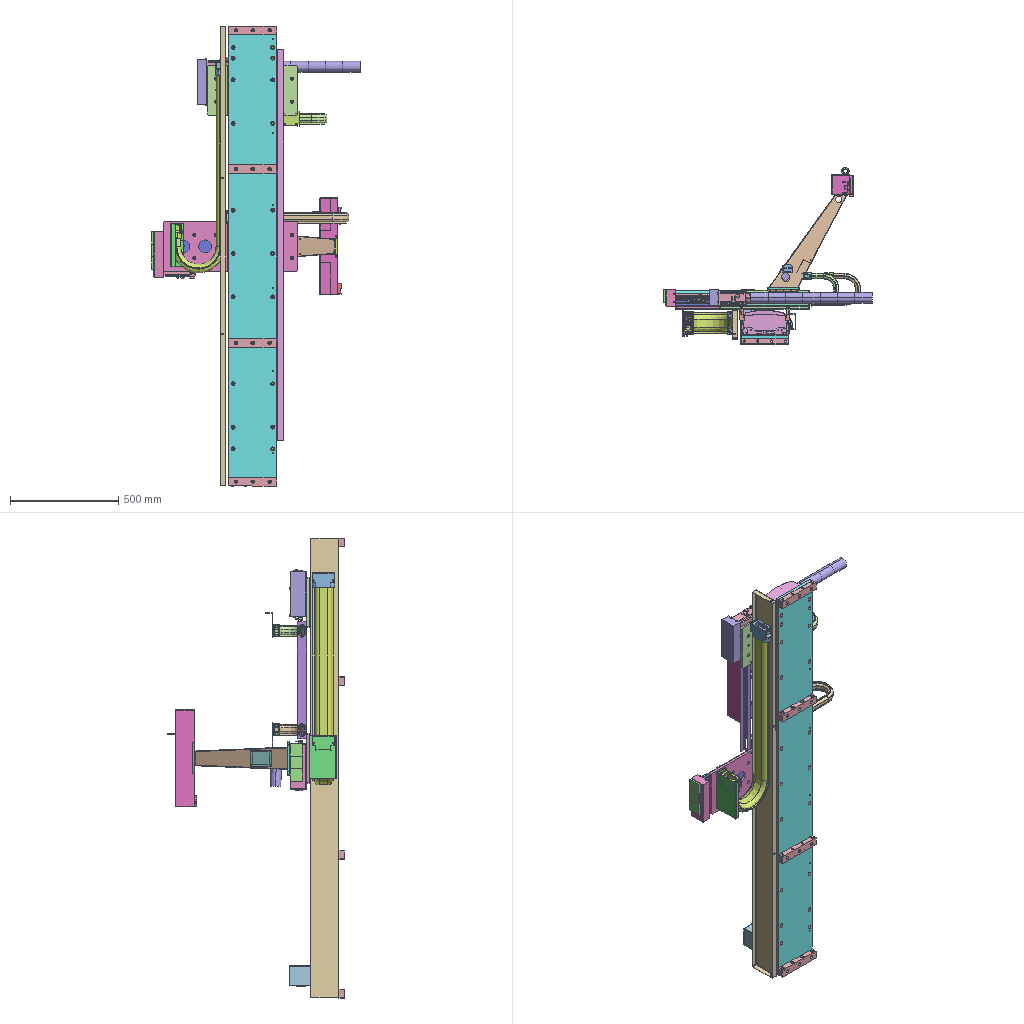Assembly | SolidWorks | 80 different items | 115 placed | box 960 x 815 x 2120 mm
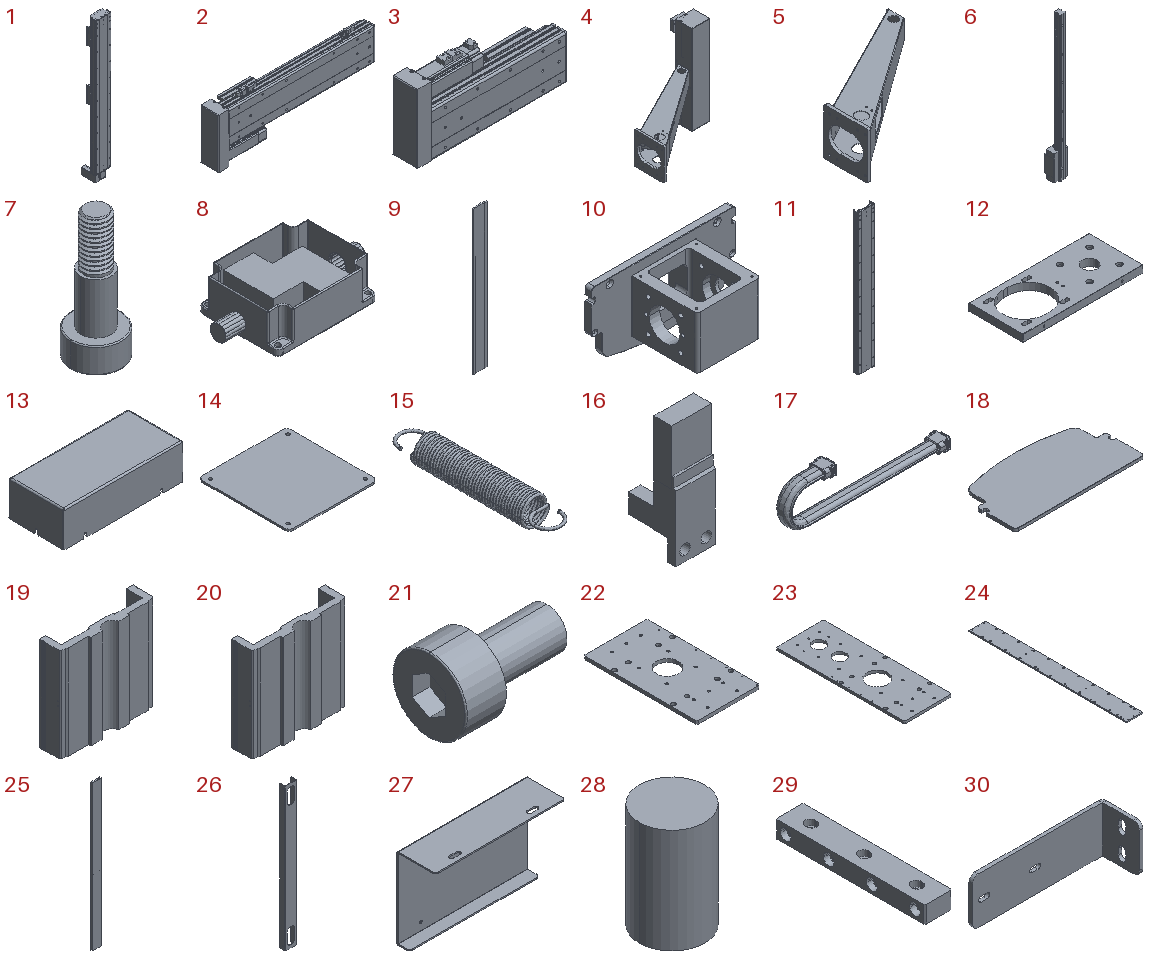Parts list (item | name | quantity | parent item | size | volume | features):
1 | (subassembly) | x1 | - | 242 x 213.35 x 2015 mm | 19740155 mm3 | -
2 | (subassembly) | x1 | - | 660 x 78 x 229.35 mm | 4358113 mm3 | -
3 | (subassembly) | x1 | - | 460 x 78 x 235.85 mm | 3440489 mm3 | -
4 | (subassembly) | x1 | - | 562.593 x 396.277 x 446 mm | 1438973 mm3 | -
5 | (subassembly) | x1 | in 4 | 438.467 x 369.277 x 160 mm | 471862 mm3 | -
6 | (subassembly) | x1 | in 4 | 34 x 28 x 350 mm | 100093 mm3 | -
7 | - | x1 | in 4 | 10 x 10 x 25 mm | 739.596 mm3 | features ICE 3, Chamfer 1, Extrusion 1, Fillet 1, SweepThread 1
8 | - | x1 | in 4 | 140 x 80 x 36 mm | 91649 mm3 | features Boss 2, Cut 2, Extrusion 1, Fillet 1, LPattern 1, Shell 1
9 | - | x1 | in 1 | 188.037 x 25 x 1900 mm | 6268934 mm3 | features BaseBody 1
10 | - | x1 | in 1 | 220 x 126 x 113.5 mm | 568343 mm3 | features BaseBody 1
11 | - | x1 | in 1 | 220 x 67.5 x 1900 mm | 10276544 mm3 | features BaseBody 1
12 | - | x1 | in 1 | 200 x 90 x 12 mm | 145701 mm3 | features BaseBody 1
13 | - | x1 | in 1 | 203.7 x 93.7 x 60.5 mm | 79662 mm3 | features BaseBody 1
14 | - | x2 | in 1 | 97 x 100 x 2 mm | 19276 mm3 | features BaseBody 1
15 | - | x1 | in 4 | 6.01 x 35.7 x 6.018 mm | 209.96 mm3 | features BaseBody 83
16 | - | x4 | in 1 | 13 x 15.5 x 39.5 mm | 3396 mm3 | features BaseBody 2
17 | - | x1 | - | 573.5 x 56 x 153.4 mm | 269954 mm3 | features BaseBody 3
18 | - | x1 | in 1 | 220 x 113.5 x 5 mm | 112175 mm3 | features BaseBody 1
19 | - | x1 | in 1 | 230 x 60 x 230 mm | 1114980 mm3 | features BaseBody 1
20 | - | x1 | in 1 | 230 x 60 x 230 mm | 1114980 mm3 | features BaseBody 1
21 | - | x14 | in 1 | 9 x 5.5 x 5.5 mm | 106.321 mm3 | features BaseBody 1
22 | - | x1 | - | 230 x 415 x 12 mm | 1051466 mm3 | features HoleWzd 5, Chamfer 1, Extrusion 1, ICE 1
23 | - | x1 | - | 230 x 616 x 12 mm | 1500608 mm3 | features HoleWzd 6, Chamfer 1, Extrusion 1, ICE 1
24 | - | x1 | - | 220 x 2115 x 15 mm | 6896303 mm3 | features HoleWzd 3, Chamfer 1, Extrusion 1
25 | - | x1 | - | 132 x 25 x 2116 mm | 573342 mm3 | features ICE 2, EdgeFlange 1, FlatPattern 1, HoleWzd 1, SMBaseFlange 1, SheetMetal 1
26 | - | x1 | - | 43 x 21.5 x 540 mm | 61599 mm3 | features Cut 1, Fillet 1, FlatPattern 1, HoleWzd 1, SMBaseFlange 1, SheetMetal 1
27 | - | x1 | - | 200 x 60 x 125 mm | 79463 mm3 | features Fillet 1, FlatPattern 1, HoleWzd 1, ICE 1, SMBaseFlange 1, SheetMetal 1
28 | - | x8 | - | 50 x 50 x 80 mm | 157080 mm3 | features Extrusion 1
29 | - | x4 | - | 40 x 220 x 25 mm | 193089 mm3 | features HoleWzd 2, Chamfer 1, Extrusion 1
30 | - | x2 | - | 115 x 35 x 40 mm | 16866 mm3 | features ICE 2, Fillet 1, FlatPattern 1, HoleWzd 1, SMBaseFlange 1, SheetMetal 1
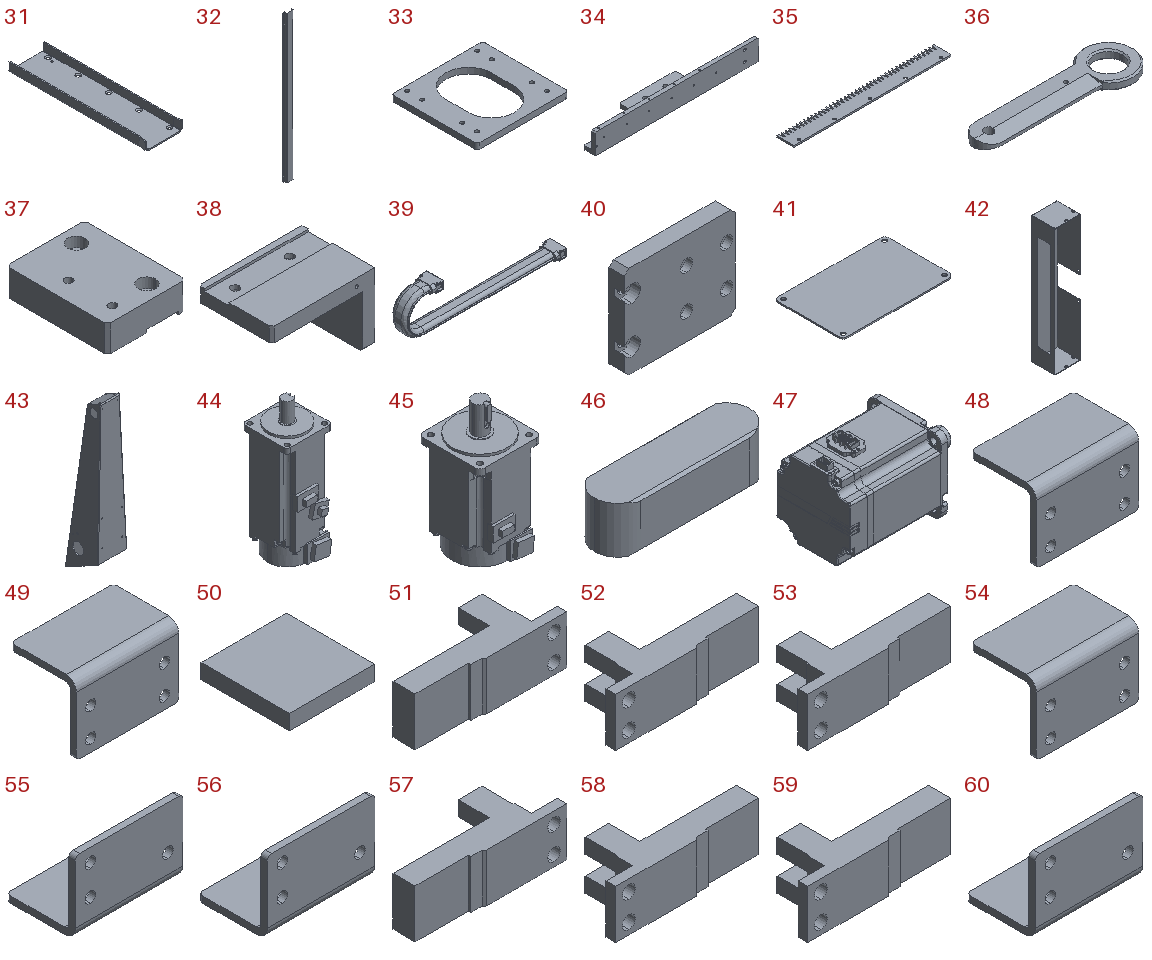31 | - | x2 | - | 69.801 x 254 x 16 mm | 45736 mm3 | features EdgeFlange 2, HoleWzd 2, Fillet 1, FlatPattern 1, ICE 1, SMBaseFlange 1, SheetMetal 1
32 | - | x1 | - | 92 x 32 x 1800 mm | 504480 mm3 | features Fillet 1, FlatPattern 1, ICE 1, SMBaseFlange 1, SheetMetal 1
33 | - | x1 | in 5 | 160 x 150 x 10 mm | 151669 mm3 | features Cut 1, Extrusion 1, Fillet 1, HoleWzd 1
34 | - | x1 | in 4 | 440 x 80 x 55 mm | 398630 mm3 | features HoleWzd 7, ICE 2, Chamfer 1, Extrusion 1, MirrorPattern 1
35 | - | x1 | in 4 | 300 x 33 x 3 mm | 24182 mm3 | features Chamfer 1, Extrusion 1, HoleWzd 1, ICE 1
36 | - | x1 | in 4 | 112.5 x 35 x 6 mm | 11153 mm3 | features ICE 3, Chamfer 1, Extrusion 1, HoleWzd 1
37 | - | x1 | in 4 | 50 x 65 x 17 mm | 50042 mm3 | features HoleWzd 2, Chamfer 1, Extrusion 1, ICE 1
38 | - | x1 | in 4 | 85 x 60 x 55 mm | 81319 mm3 | features HoleWzd 5, ICE 4, Chamfer 2, Extrusion 1
39 | - | x1 | - | 978 x 104 x 250 mm | 1591842 mm3 | features BaseBody 3, ICE 1
40 | - | x1 | in 4 | 72 x 10 x 60 mm | 39992 mm3 | features HoleWzd 4, Chamfer 2, Extrusion 1, ICE 1
41 | - | x1 | in 4 | 120 x 75 x 1.5 mm | 13372 mm3 | features Fillet 1, FlatPattern 1, HoleWzd 1, SMBaseFlange 1, SheetMetal 1
42 | - | x1 | in 4 | 91 x 82 x 446 mm | 155012 mm3 | features Cut 4, EdgeFlange 1, Fillet 1, FlatPattern 1, SMBaseFlange 1, SheetMetal 1
43 | - | x1 | in 5 | 103.468 x 118.808 x 550 mm | 320193 mm3 | features HoleWzd 4, Fillet 3, Cut 2, ICE 2, Blend 1, MirrorPattern 1, Shell 1
44 | - | x2 | - | 60.07 x 70.835 x 176.5 mm | 467589 mm3 | features BaseBody 1, ICE 1
45 | - | x1 | - | 80.44 x 89.02 x 162.2 mm | 690586 mm3 | features BaseBody 1, ICE 1, MoveCopyBody 1, Stock 1
46 | - | x1 | - | 20 x 6 x 6 mm | 670.871 mm3 | features Extrusion 1, ICE 1
47 | - | x1 | in 1 | - | - | features BaseBody 55, RefSurface 21
48 | - | x1 | in 3 | 25 x 16 x 17 mm | 1122 mm3 | features BaseBody 1
49 | - | x1 | in 3 | 25 x 16 x 17 mm | 1122 mm3 | features BaseBody 1
50 | - | x3 | - | 56.969 x 58.85 x 10 mm | 33526 mm3 | features Extrusion 1
51 | - | x1 | in 3 | 39.5 x 15.5 x 13 mm | 3385 mm3 | features BaseBody 1
52 | - | x1 | in 3 | 39.5 x 15.5 x 13 mm | 3385 mm3 | features BaseBody 1
53 | - | x1 | in 3 | 39.5 x 15.5 x 13 mm | 3385 mm3 | features BaseBody 1
54 | - | x1 | in 3 | 25 x 16 x 17 mm | 1122 mm3 | features BaseBody 1
55 | - | x1 | in 2 | 25 x 16 x 17 mm | 1130 mm3 | features BaseBody 1
56 | - | x1 | in 2 | 25 x 16 x 17 mm | 1130 mm3 | features BaseBody 1
57 | - | x1 | in 2 | 39.5 x 15.5 x 13 mm | 3385 mm3 | features BaseBody 1
58 | - | x1 | in 2 | 39.5 x 15.5 x 13 mm | 3385 mm3 | features BaseBody 1
59 | - | x1 | in 2 | 39.5 x 15.5 x 13 mm | 3385 mm3 | features BaseBody 1
60 | - | x1 | in 2 | 25 x 16 x 17 mm | 1130 mm3 | features BaseBody 1
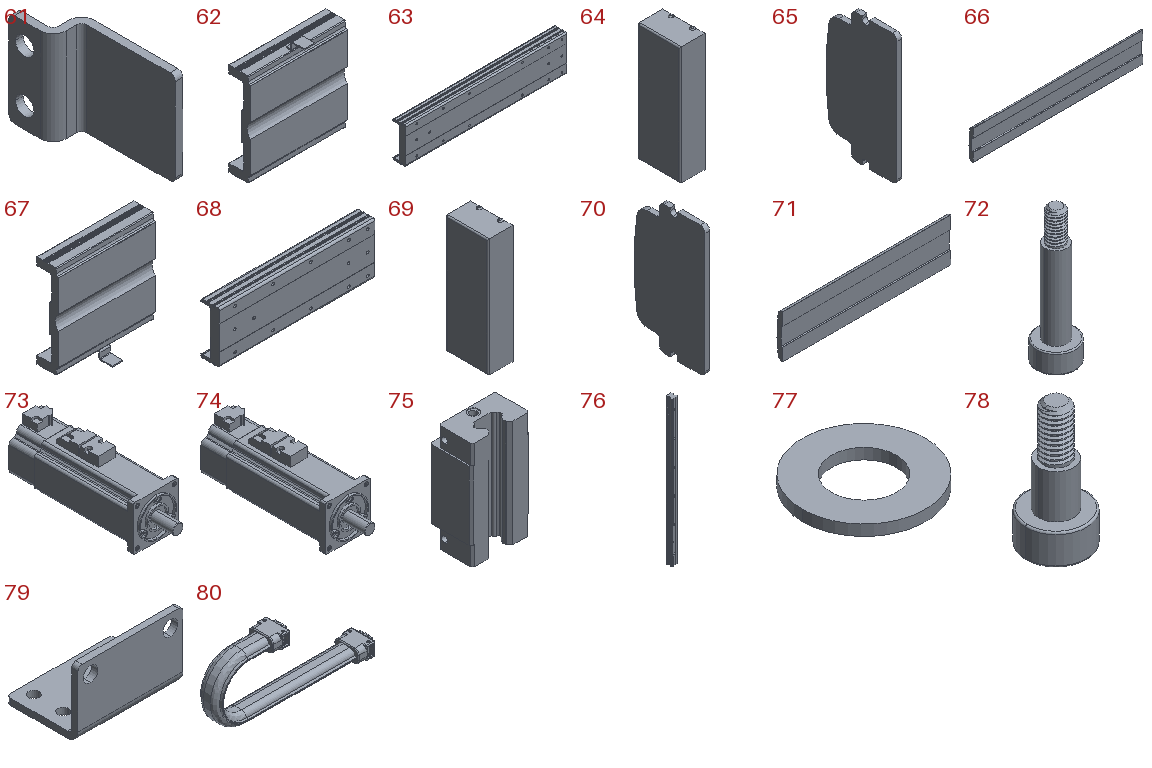61 | - | x1 | in 1 | 7 x 26.5 x 18 mm | 793.289 mm3 | features BaseBody 1
62 | - | x1 | in 2 | 140 x 47 x 146 mm | 250263 mm3 | features BaseBody 1
63 | - | x1 | in 2 | 611 x 48 x 135 mm | 2089073 mm3 | features BaseBody 1
64 | - | x1 | in 2 | 44 x 75.3 x 214.7 mm | 696283 mm3 | features BaseBody 1
65 | - | x1 | in 2 | 5 x 74 x 135 mm | 44638 mm3 | features BaseBody 1
66 | - | x1 | in 2 | 611 x 14.5 x 106.047 mm | 703193 mm3 | features BaseBody 1
67 | - | x1 | in 3 | 140 x 47 x 146 mm | 250263 mm3 | features BaseBody 1
68 | - | x1 | in 3 | 411 x 48 x 135 mm | 1401649 mm3 | features BaseBody 1
69 | - | x1 | in 3 | 44 x 75.3 x 214.7 mm | 696283 mm3 | features BaseBody 1
70 | - | x1 | in 3 | 5 x 74 x 135 mm | 44638 mm3 | features BaseBody 1
71 | - | x1 | in 3 | 411 x 14.5 x 106.047 mm | 473016 mm3 | features BaseBody 1
72 | - | x1 | in 4 | 7 x 7 x 24.2 mm | 319.419 mm3 | features ICE 3, Chamfer 1, Extrusion 1, Fillet 1, SweepThread 1
73 | - | x1 | in 3 | 60 x 196.8 x 72.85 mm | 561117 mm3 | features BaseBody 1
74 | - | x1 | in 2 | 60 x 196.8 x 72.85 mm | 561117 mm3 | features BaseBody 1
75 | - | x1 | in 6 | 34 x 23.7 x 61.4 mm | 36561 mm3 | features BaseBody 1
76 | - | x1 | in 6 | 15 x 15 x 350 mm | 63532 mm3 | features BaseBody 1
77 | - | x1 | in 4 | 16 x 16 x 1.4 mm | 203.902 mm3 | features Extrusion 1, RefAxis 1
78 | - | x1 | in 4 | 7 x 7 x 14.2 mm | 193.763 mm3 | features ICE 3, Chamfer 1, Extrusion 1, Fillet 1, SweepThread 1
79 | - | x4 | in 1 | 25 x 17 x 16 mm | 1093 mm3 | features BaseBody 1
80 | - | x1 | - | 373.5 x 56 x 153.4 mm | 213102 mm3 | features BaseBody 3
Mates (type | each side: item.copy, entity, surface, feature):
In the top assembly
Coincident | 24.1 face plane Boss-Extrude 1 | 29.1 face plane Boss-Extrude 1
Width | 29.1 face plane Boss-Extrude 1 | 29.1 face plane Boss-Extrude 1 | 24.1 face plane Boss-Extrude 1 | 24.1 face plane Boss-Extrude 1
DistanceDim | 24.1 face plane Boss-Extrude 1 | 29.1 face plane Boss-Extrude 1
Coincident | 24.1 face plane Boss-Extrude 1 | 29.2 face plane Boss-Extrude 1 | 2 times
DistanceDim | 29.3 face plane Boss-Extrude 1 | 24.1 face plane Boss-Extrude 1
DistanceDim | 29.4 face plane Boss-Extrude 1 | 29.1 face plane Boss-Extrude 1
DistanceDim | 29.2 face plane Boss-Extrude 1 | 29.3 face plane Boss-Extrude 1
Coincident | 24.1 face plane Boss-Extrude 1 | 29.4 face plane Boss-Extrude 1 | 2 times
Coincident | 24.1 face plane Boss-Extrude 1 | 29.3 face plane Boss-Extrude 1 | 2 times
Coincident | 22.1 face plane Boss-Extrude 1 | 68.1 face plane Input 1
Coincident | 22.1 face plane Boss-Extrude 1 | 70.1 face plane Input 1
Coincident | 23.1 face plane Boss-Extrude 1 | 63.1 face plane Input 1
Coincident | 23.1 face plane Boss-Extrude 1 | 65.1 face plane Input 1
Coincident | 33.1 face plane Boss-Extrude 1 | 62.1 face plane Input 1 | 2 times
Width | 33.1 face plane Boss-Extrude 1 | 33.1 face plane Boss-Extrude 1 | 62.1 face plane Input 1 | 62.1 face plane Input 1
Coincident | 22.1 face plane Boss-Extrude 1 | 23.1 face plane Boss-Extrude 1
Coincident | 38.1 face plane Cut-Extrude 1 | assembly face | 2 times
Width | assembly face | assembly face | 37.1 face plane Boss-Extrude 1 | 37.1 face plane Boss-Extrude 1
Coincident | 37.1 face plane Cut-Extrude 1 | assembly face
Width | 69.1 face plane Input 1 | 70.1 face plane Input 1 | 80.1 face plane 2025_12_29_09_47_18_0776-1-solid1 | 80.1 face plane 2025_12_29_09_47_18_0776-1-solid1
Coincident | 30.1 face plane Base-Flange 1 | 80.1 face plane 2025_12_29_09_47_18_0791-1-solid1
Coincident | 30.1 face plane Base-Flange 1 | 30.2 face plane Base-Flange 1
Coincident | 80.1 face plane 2025_12_29_09_47_18_0791-1-solid1 | 17.1 face plane 2025_12_29_10_27_39_0817-1-solid1
Width | 64.1 face plane Input 1 | 65.1 face plane Input 1 | 17.1 face plane 2025_12_29_10_27_39_0801-1-solid1 | 17.1 face plane 2025_12_29_10_27_39_0801-1-solid1
DistanceDim | 30.2 face plane Base-Flange 1 | 33.1 face plane Boss-Extrude 1 | 2 times
DistanceDim | 30.1 face plane Base-Flange 1 | 80.1 face plane 2025_12_29_09_47_18_0791-1-solid1
DistanceDim | 17.1 face plane 2025_12_29_10_27_39_0817-1-solid1 | 30.2 face plane Base-Flange 1
DistanceDim | 80.1 face plane 2025_12_29_09_47_18_0776-1-solid1 | 22.1 face plane Boss-Extrude 1
Coincident | 22.1 face plane Boss-Extrude 1 | 26.1 face plane Base-Flange 1
DistanceDim | 26.1 face plane Base-Flange 1 | 17.1 face plane 2025_12_29_10_27_39_0801-1-solid1
DistanceDim | 26.1 face plane Base-Flange 1 | 23.1 face plane Boss-Extrude 1
Parallel | 23.1 face plane Boss-Extrude 1 | 25.1 face plane Edge-Flange 2
Width | 25.1 face plane Edge-Flange 2 | 25.1 face plane Edge-Flange 2 | 24.1 face plane Boss-Extrude 1 | 24.1 face plane Boss-Extrude 1
Coincident | 24.1 face plane Boss-Extrude 1 | 11.1 face plane Input 1
Width | 11.1 face plane Input 1 | 11.1 face plane Input 1 | 24.1 face plane Boss-Extrude 1 | 24.1 face plane Boss-Extrude 1
DistanceDim | 18.1 face plane Input 1 | 24.1 face plane Boss-Extrude 1
Coincident | 22.1 face plane Boss-Extrude 1 | 20.1 face plane Input 1
Width | 22.1 face plane Boss-Extrude 1 | 22.1 face plane Boss-Extrude 1 | 20.1 face plane Input 1 | 20.1 face plane Input 1
DistanceDim | 20.1 face plane Input 1 | 22.1 face plane Boss-Extrude 1
Width | 68.1 face plane Input 1 | 68.1 face plane Input 1 | 22.1 face plane Boss-Extrude 1 | 22.1 face plane Boss-Extrude 1
Width | 63.1 face plane Input 1 | 63.1 face plane Input 1 | 23.1 face plane Boss-Extrude 1 | 23.1 face plane Boss-Extrude 1
Width | 23.1 face plane Boss-Extrude 1 | 23.1 face plane Boss-Extrude 1 | 19.1 face plane Input 1 | 19.1 face plane Input 1
Coincident | 23.1 face plane Boss-Extrude 1 | 19.1 face plane Input 1
Coincident | 80.1 face plane 2025_12_29_09_47_18_0791-1-solid1 | assembly face | 2 times
Slot | assembly face | 30.1 face cylinder Cut-Extrude 1
Coincident | 17.1 face plane 2025_12_29_10_27_39_0817-1-solid1 | assembly face | 2 times
Slot | assembly face | 30.2 face cylinder Cut-Extrude 1
Coincident | 22.1 face plane Boss-Extrude 1 | 31.1 face plane Base-Flange 1
Width | 31.1 face plane Edge-Flange 1 | 31.1 face plane Edge-Flange 1 | 80.1 face plane 2025_12_29_09_47_18_0776-1-solid1 | 80.1 face plane 2025_12_29_09_47_18_0776-1-solid1
Coincident | 23.1 face plane Boss-Extrude 1 | 31.2 face plane Base-Flange 1
Width | 31.2 face plane Edge-Flange 1 | 31.2 face plane Edge-Flange 1 | 17.1 face plane 2025_12_29_10_27_39_0801-1-solid1 | 17.1 face plane 2025_12_29_10_27_39_0801-1-solid1
DistanceDim | 31.2 face plane Edge-Flange 1 | 26.1 face plane Base-Flange 1
DistanceDim | 25.1 face plane Base-Flange 1 | 20.1 face plane Input 1
Coincident | 11.1 face plane Input 1 | 32.1 face plane Base-Flange 1
Width | 10.1 face plane Input 1 | 18.1 face plane Input 1 | 32.1 face plane Base-Flange 1 | 32.1 face plane Base-Flange 1
DistanceDim | 24.1 face plane Boss-Extrude 1 | 32.1 face plane Base-Flange 1
Coincident | 73.1 face plane Input 1 | 44.1 face plane Input 1
Concentric | 73.1 face cylinder Input 1 | 44.1 face cylinder Input 1
Parallel | 69.1 face plane Input 1 | 44.1 face plane Input 1
Coincident | 74.1 face plane Input 1 | 44.2 face plane Input 1
Concentric | 74.1 face cylinder Input 1 | 44.2 face cylinder Input 1
Parallel | 64.1 face plane Input 1 | 44.2 face plane Input 1
Coincident | 25.1 face plane Base-Flange 1 | 39.1 face plane 2026_01_05_13_31_16_0000-1-solid1
Coincident | 27.1 face plane Base-Flange 1 | 39.1 face plane 2026_01_05_13_31_15_0984-1-solid1 | 2 times
DistanceDim | 27.1 face plane Base-Flange 1 | 23.1 face plane Boss-Extrude 1
Coincident | 23.1 face plane Boss-Extrude 1 | 27.1 face plane Base-Flange 1
Coincident | 24.1 face plane Boss-Extrude 1 | 25.1 face plane Edge-Flange 2
Concentric | 39.1 face cylinder 2026_01_05_13_31_15_0984-1-solid1 | 27.1 face cylinder M5 Tapped Hole 1
Coincident | 12.1 face plane Input 1 | 45.1 face plane Input 1
Slot | 45.1 face cylinder Input 1 | 12.1 face cylinder Input 1
Parallel | 13.1 face plane Input 1 | 45.1 face plane Input 1
Coincident | 67.1 face plane Input 1 | assembly face | 2 times
Width | assembly face | assembly face | 67.1 face plane Input 1 | 67.1 face plane Input 1 | 2 times
Concentric | 67.1 face cylinder Input 1 | assembly face | 2 times
Concentric | 22.1 face cylinder M4 Tapped Hole 1 | 31.1 face cone M4 Hex Socket Cone Point Set Screw Countersink Hole 1
DistanceDim | 30.1 face plane Base-Flange 1 | assembly face
Coincident | 43.1 face plane Loft 2 | 28.1 face plane Boss-Extrude 1
Concentric | 43.1 face cylinder Cut-Extrude 14 | 28.1 face cylinder Boss-Extrude 1
Coincident | 44.1 face plane Input 1 | 28.2 face plane Boss-Extrude 1
Concentric | 44.1 face cylinder Input 1 | 28.2 face cylinder Boss-Extrude 1
Coincident | 28.2 face plane Boss-Extrude 1 | 28.3 face plane Boss-Extrude 1
Concentric | 28.2 face cylinder Boss-Extrude 1 | 28.3 face cylinder Boss-Extrude 1
Coincident | 28.3 face plane Boss-Extrude 1 | 28.4 face plane Boss-Extrude 1
Concentric | 28.3 face cylinder Boss-Extrude 1 | 28.4 face cylinder Boss-Extrude 1
Coincident | 64.1 face plane Input 1 | 50.1 face plane Boss-Extrude 1 | 3 times
Coincident | 64.1 face plane Input 1 | 50.2 face plane Boss-Extrude 1 | 2 times
Coincident | 50.1 face plane Boss-Extrude 1 | 50.2 face plane Boss-Extrude 1
Coincident | 64.1 face plane Input 1 | 50.3 face plane Boss-Extrude 1 | 2 times
Coincident | 50.2 face plane Boss-Extrude 1 | 50.3 face plane Boss-Extrude 1
In subassembly 4
Coincident | 33.2 face plane Boss-Extrude 1 | 4.1 plane | 3 times
Width | 34.1 face plane Boss-Extrude 1 | 34.1 face plane Boss-Extrude 1 | 33.2 face plane Boss-Extrude 1 | 33.2 face plane Boss-Extrude 1
Coincident | 76.1 face plane Input 1 | 34.1 face plane Boss-Extrude 2
Coincident | 34.1 face plane Boss-Extrude 1 | 35.1 face plane Boss-Extrude 1 | 2 times
Coincident | 76.1 face plane Input 1 | 34.1 face plane Boss-Extrude 1
Coincident | 34.1 face plane Boss-Extrude 1 | 37.2 face plane Boss-Extrude 1 | 2 times
Coincident | 34.1 face plane Boss-Extrude 2 | 37.2 face plane Boss-Extrude 1
DistanceDim | 38.2 face plane Boss-Extrude 1 | 34.1 face plane Boss-Extrude 1
Coincident | 34.1 face plane Boss-Extrude 1 | 38.2 face plane Boss-Extrude 1
Coincident | 38.2 face plane Boss-Extrude 1 | 40.1 face plane Boss-Extrude 1
Width | 40.1 face plane Boss-Extrude 1 | 40.1 face plane Boss-Extrude 1 | 75.1 face plane Input 1 | 75.1 face plane Input 1
Coincident | 34.1 face plane Boss-Extrude 2 | 35.1 face plane Boss-Extrude 1
Width | 43.2 face plane Loft 2 | 43.2 face plane Loft 2 | 8.1 face plane Extrude 1 | 8.1 face plane Extrude 1
Concentric | 36.1 face cylinder Boss-Extrude 3 | 40.1 face cylinder M6 Tapped Hole 2
Concentric | 40.1 face cylinder M6 Tapped Hole 2 | 7.1 face cylinder Boss-Extrude 2
Coincident | 36.1 face plane Boss-Extrude 3 | 7.1 face plane Boss-Extrude 1
Coincident | 40.1 face plane Boss-Extrude 1 | 7.1 face plane Boss-Extrude 2
Width | 42.1 face plane Base-Flange 1 | 42.1 face plane Base-Flange 1 | 34.1 face plane Boss-Extrude 1 | 34.1 face plane Boss-Extrude 1
DistanceDim | 43.2 face plane Boss-Extrude 9 | 34.1 face plane Boss-Extrude 1
Coincident | 43.2 face plane Shell 1 | 8.1 face plane Extrude 1
DistanceDim | 33.2 edge | 8.1 face plane Extrude 1
Coincident | 43.2 face plane Loft 2 | 41.1 face plane Base-Flange 1
Width | 41.1 face plane Base-Flange 1 | 41.1 face plane Base-Flange 1 | 43.2 face plane Cut-Extrude 16 | 43.2 face plane Cut-Extrude 16
Width | 43.2 face plane Cut-Extrude 16 | 43.2 face plane Cut-Extrude 16 | 41.1 face plane Base-Flange 1 | 41.1 face plane Base-Flange 1
Coincident | 34.1 face plane Boss-Extrude 1 | 42.1 face plane Base-Flange 1
Concentric | 7.1 face cylinder Boss-Extrude 2 | 77.1 face cylinder Boss-Extrude 1
Coincident | 40.1 face plane Boss-Extrude 1 | 77.1 face plane Boss-Extrude 1
Coincident | 35.1 edge | 36.1 face plane Boss-Extrude 3
Slot | 42.1 face cylinder Cut-Extrude 3 | 34.1 face cylinder Mirror 1
Concentric | 76.1 face cylinder Input 1 | 34.1 face cylinder M4 Tapped Hole 1
Coincident | 43.2 face plane Cut-Extrude 13 | 34.1 face plane Boss-Extrude 1
Coincident | 72.1 face plane Boss-Extrude 1 | 78.1 face plane Boss-Extrude 1
DistanceDim | 15.1 plane | 78.1 plane | 2 times
Coincident | 15.1 plane | 78.1 plane
Concentric | 36.1 face cylinder M3 Tapped Hole 1 | 78.1 face cylinder Boss-Extrude 2
Coincident | 36.1 face plane Boss-Extrude 3 | 78.1 face plane Boss-Extrude 2
Concentric | 38.2 face cylinder M3 Tapped Hole 1 | 72.1 face cylinder Boss-Extrude 2
Coincident | 15.1 plane | 72.1 plane
Coincident | 38.2 face plane Boss-Extrude 2 | 40.1 face plane Boss-Extrude 1 | 2 times
In subassembly 5
Coincident | 33.3 face plane Boss-Extrude 1 | 43.3 face plane Cut-Extrude 13
Width | 33.3 face plane Boss-Extrude 1 | 33.3 face plane Boss-Extrude 1 | 43.3 face plane Loft 2 | 43.3 face plane Loft 2
DistanceDim | 43.3 edge | 33.3 face plane Boss-Extrude 1
In subassembly 6
LimitDistanceDim | 75.2 face plane Input 1 | 76.2 face plane Input 1
Coincident | 75.2 face plane Input 1 | 76.2 face plane Input 1
Width | 76.2 face plane Input 1 | 76.2 face plane Input 1 | 75.2 face plane Input 1 | 75.2 face plane Input 1
In subassembly 1
DistanceDim | 20.2 face plane Input 1 | 19.2 face plane Input 1
Coincident | 19.2 face plane Input 1 | 20.2 face plane Input 1 | 2 times
DistanceDim | 19.2 face plane Input 1 | 13.2 face plane Input 1
DistanceDim | 13.2 face plane Input 1 | 19.2 face plane Input 1
LimitDistanceDim | 19.2 face plane Input 1 | 13.2 face plane Input 1
In subassembly 2
DistanceDim | 62.2 face plane Input 1 | 64.2 face plane Input 1 | 2 times
LimitDistanceDim | 64.2 face plane Input 1 | 62.2 face plane Input 1
In subassembly 3
DistanceDim | 67.2 face plane Input 1 | 69.2 face plane Input 1 | 2 times
LimitDistanceDim | 67.2 face plane Input 1 | 69.2 face plane Input 1